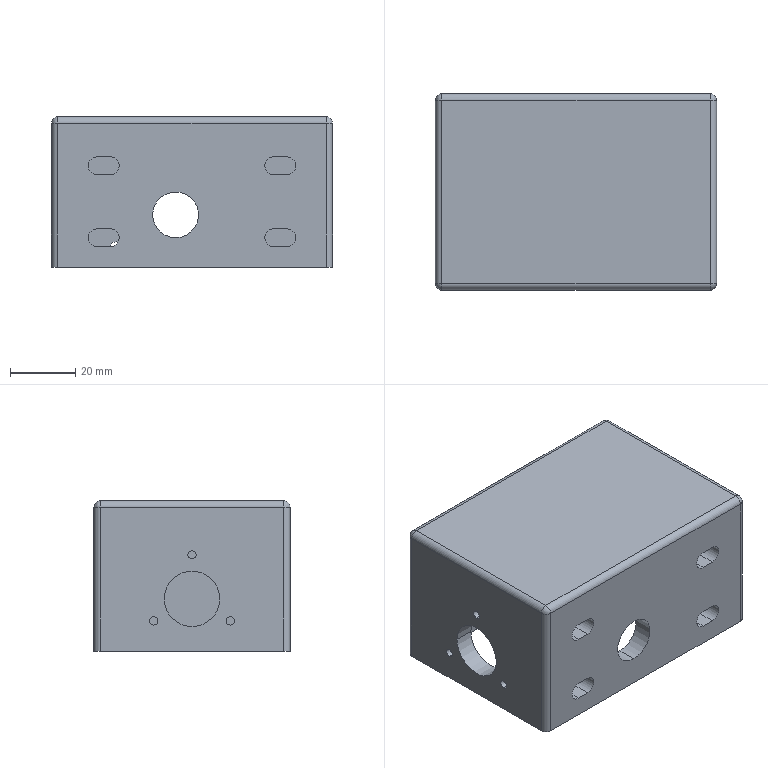Part | SolidWorks | features ICE 4, 3DProfileFeature 2, Fillet 2, HoleWzd 2, Extrusion 1 | 1 solid | 77 faces | box 86 x 60 x 46 mm | volume 87351 mm3 | cylinder 46 | plane 19 | cone 8 | sphere 4 | commonest cylinder face diameters 2.5 x14 4 x8 5.5 x8 4.5 x6 10 x4 14 x4